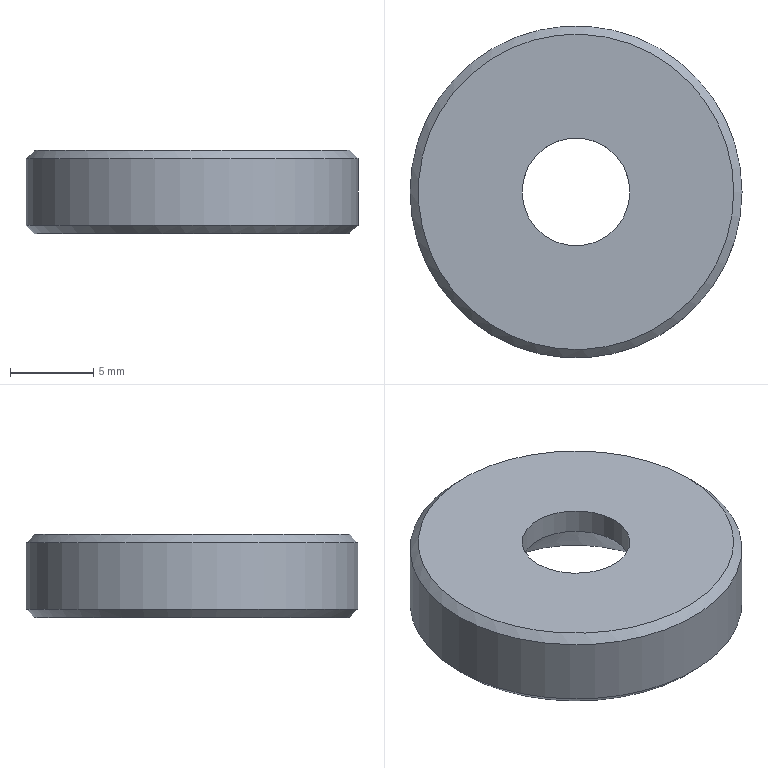Part | STEP file | LJD_id166_x_t | 1 solid | 7 faces | box 20 x 20 x 5 mm | volume 1219 mm3 | cone 3 | plane 2 | cylinder 2 | commonest cylinder face diameters 6.5 x1 20 x1
STEP:
#1=CARTESIAN_POINT('',(45.5,0.,-165.5));
#2=VERTEX_POINT('',#1);
#3=CARTESIAN_POINT('',(55.,0.,-165.5));
#4=DIRECTION('',(0.,0.,-1.));
#5=DIRECTION('',(-1.,0.,0.));
#6=AXIS2_PLACEMENT_3D('',#3,#4,#5);
#7=CIRCLE('',#6,9.5);
#8=EDGE_CURVE('',#2,#2,#7,.T.);
#9=ORIENTED_EDGE('',*,*,#8,.T.);
#10=EDGE_LOOP('',(#9));
#11=FACE_BOUND('',#10,.T.);
#12=CARTESIAN_POINT('',(61.75,0.,-165.5));
#13=VERTEX_POINT('',#12);
#14=CARTESIAN_POINT('',(55.,0.,-165.5));
#15=DIRECTION('',(0.,0.,1.));
#16=DIRECTION('',(1.,0.,0.));
#17=AXIS2_PLACEMENT_3D('',#14,#15,#16);
#18=CIRCLE('',#17,6.75);
#19=EDGE_CURVE('',#13,#13,#18,.T.);
#20=ORIENTED_EDGE('',*,*,#19,.T.);
#21=EDGE_LOOP('',(#20));
#22=FACE_BOUND('',#21,.T.);
#23=CARTESIAN_POINT('',(55.,0.,-165.5));
#24=DIRECTION('',(0.,0.,-1.));
#25=DIRECTION('',(-1.,0.,0.));
#26=AXIS2_PLACEMENT_3D('',#23,#24,#25);
#27=PLANE('',#26);
#28=ADVANCED_FACE('',(#11,#22),#27,.T.);
#29=CARTESIAN_POINT('',(64.5,0.,-160.5));
#30=VERTEX_POINT('',#29);
#31=CARTESIAN_POINT('',(55.,0.,-160.5));
#32=DIRECTION('',(0.,0.,1.));
#33=DIRECTION('',(1.,0.,0.));
#34=AXIS2_PLACEMENT_3D('',#31,#32,#33);
#35=CIRCLE('',#34,9.5);
#36=EDGE_CURVE('',#30,#30,#35,.T.);
#37=ORIENTED_EDGE('',*,*,#36,.T.);
#38=EDGE_LOOP('',(#37));
#39=FACE_BOUND('',#38,.T.);
#40=CARTESIAN_POINT('',(58.25,0.,-160.5));
#41=VERTEX_POINT('',#40);
#42=CARTESIAN_POINT('',(55.,0.,-160.5));
#43=DIRECTION('',(0.,0.,1.));
#44=DIRECTION('',(1.,0.,0.));
#45=AXIS2_PLACEMENT_3D('',#42,#43,#44);
#46=CIRCLE('',#45,3.25);
#47=EDGE_CURVE('',#41,#41,#46,.T.);
#48=ORIENTED_EDGE('',*,*,#47,.F.);
#49=EDGE_LOOP('',(#48));
#50=FACE_BOUND('',#49,.T.);
#51=CARTESIAN_POINT('',(55.,0.,-160.5));
#52=DIRECTION('',(0.,0.,1.));
#53=DIRECTION('',(1.,0.,0.));
#54=AXIS2_PLACEMENT_3D('',#51,#52,#53);
#55=PLANE('',#54);
#56=ADVANCED_FACE('',(#39,#50),#55,.T.);
#57=CARTESIAN_POINT('',(65.,0.,-161.));
#58=VERTEX_POINT('',#57);
#59=CARTESIAN_POINT('',(55.,0.,-161.));
#60=DIRECTION('',(0.,0.,-1.));
#61=DIRECTION('',(1.,0.,0.));
#62=AXIS2_PLACEMENT_3D('',#59,#60,#61);
#63=CIRCLE('',#62,10.);
#64=EDGE_CURVE('',#58,#58,#63,.T.);
#65=ORIENTED_EDGE('',*,*,#64,.T.);
#66=EDGE_LOOP('',(#65));
#67=FACE_BOUND('',#66,.T.);
#68=CARTESIAN_POINT('',(45.,0.,-165.));
#69=VERTEX_POINT('',#68);
#70=CARTESIAN_POINT('',(55.,0.,-165.));
#71=DIRECTION('',(0.,0.,1.));
#72=DIRECTION('',(-1.,0.,0.));
#73=AXIS2_PLACEMENT_3D('',#70,#71,#72);
#74=CIRCLE('',#73,10.);
#75=EDGE_CURVE('',#69,#69,#74,.T.);
#76=ORIENTED_EDGE('',*,*,#75,.T.);
#77=EDGE_LOOP('',(#76));
#78=FACE_BOUND('',#77,.T.);
#79=CARTESIAN_POINT('',(55.,0.,-165.5));
#80=DIRECTION('',(0.,0.,1.));
#81=DIRECTION('',(1.,0.,0.));
#82=AXIS2_PLACEMENT_3D('',#79,#80,#81);
#83=CYLINDRICAL_SURFACE('',#82,10.);
#84=ADVANCED_FACE('',(#67,#78),#83,.T.);
#85=CARTESIAN_POINT('',(51.75,0.,-162.));
#86=VERTEX_POINT('',#85);
#87=CARTESIAN_POINT('',(55.,0.,-162.));
#88=DIRECTION('',(0.,0.,-1.));
#89=DIRECTION('',(-1.,0.,0.));
#90=AXIS2_PLACEMENT_3D('',#87,#88,#89);
#91=CIRCLE('',#90,3.25);
#92=EDGE_CURVE('',#86,#86,#91,.T.);
#93=ORIENTED_EDGE('',*,*,#92,.T.);
#94=EDGE_LOOP('',(#93));
#95=FACE_BOUND('',#94,.T.);
#96=ORIENTED_EDGE('',*,*,#47,.T.);
#97=EDGE_LOOP('',(#96));
#98=FACE_BOUND('',#97,.T.);
#99=CARTESIAN_POINT('',(55.,0.,-165.5));
#100=DIRECTION('',(0.,0.,1.));
#101=DIRECTION('',(1.,0.,0.));
#102=AXIS2_PLACEMENT_3D('',#99,#100,#101);
#103=CYLINDRICAL_SURFACE('',#102,3.25);
#104=ADVANCED_FACE('',(#95,#98),#103,.F.);
#105=ORIENTED_EDGE('',*,*,#19,.F.);
#106=EDGE_LOOP('',(#105));
#107=FACE_BOUND('',#106,.T.);
#108=ORIENTED_EDGE('',*,*,#92,.F.);
#109=EDGE_LOOP('',(#108));
#110=FACE_BOUND('',#109,.T.);
#111=CARTESIAN_POINT('',(55.,0.,-162.));
#112=DIRECTION('',(0.,0.,-1.));
#113=DIRECTION('',(-1.,0.,0.));
#114=AXIS2_PLACEMENT_3D('',#111,#112,#113);
#115=CONICAL_SURFACE('',#114,3.25,45.);
#116=ADVANCED_FACE('',(#107,#110),#115,.F.);
#117=ORIENTED_EDGE('',*,*,#36,.F.);
#118=EDGE_LOOP('',(#117));
#119=FACE_BOUND('',#118,.T.);
#120=ORIENTED_EDGE('',*,*,#64,.F.);
#121=EDGE_LOOP('',(#120));
#122=FACE_BOUND('',#121,.T.);
#123=CARTESIAN_POINT('',(55.,0.,-161.));
#124=DIRECTION('',(0.,0.,-1.));
#125=DIRECTION('',(-1.,0.,0.));
#126=AXIS2_PLACEMENT_3D('',#123,#124,#125);
#127=CONICAL_SURFACE('',#126,10.,45.);
#128=ADVANCED_FACE('',(#119,#122),#127,.T.);
#129=ORIENTED_EDGE('',*,*,#8,.F.);
#130=EDGE_LOOP('',(#129));
#131=FACE_BOUND('',#130,.T.);
#132=ORIENTED_EDGE('',*,*,#75,.F.);
#133=EDGE_LOOP('',(#132));
#134=FACE_BOUND('',#133,.T.);
#135=CARTESIAN_POINT('',(55.,0.,-165.));
#136=DIRECTION('',(0.,0.,1.));
#137=DIRECTION('',(1.,0.,0.));
#138=AXIS2_PLACEMENT_3D('',#135,#136,#137);
#139=CONICAL_SURFACE('',#138,10.,45.);
#140=ADVANCED_FACE('',(#131,#134),#139,.T.);
#141=CLOSED_SHELL('',(#28,#56,#84,#104,#116,#128,#140));
#142=MANIFOLD_SOLID_BREP('',#141);
#143=(LENGTH_UNIT()NAMED_UNIT(*)SI_UNIT(.MILLI.,.METRE.));
#144=UNCERTAINTY_MEASURE_WITH_UNIT(LENGTH_MEASURE(0.00002),#143,'','');
#145=(NAMED_UNIT(*)PLANE_ANGLE_UNIT()SI_UNIT($,.RADIAN.));
#146=PLANE_ANGLE_MEASURE_WITH_UNIT(PLANE_ANGLE_MEASURE(0.01745),#145);
#147=DIMENSIONAL_EXPONENTS(0.,0.,0.,0.,0.,0.,0.);
#148=(CONVERSION_BASED_UNIT('DEGREE',#146)NAMED_UNIT(#147)PLANE_ANGLE_UNIT());
#149=(NAMED_UNIT(*)SI_UNIT($,.STERADIAN.)SOLID_ANGLE_UNIT());
#150=(GEOMETRIC_REPRESENTATION_CONTEXT(3)GLOBAL_UNCERTAINTY_ASSIGNED_CONTEXT((#144))GLOBAL_UNIT_ASSIGNED_CONTEXT((#143,#148,#149))REPRESENTATION_CONTEXT('',''));
#151=ADVANCED_BREP_SHAPE_REPRESENTATION('',(#142),#150);